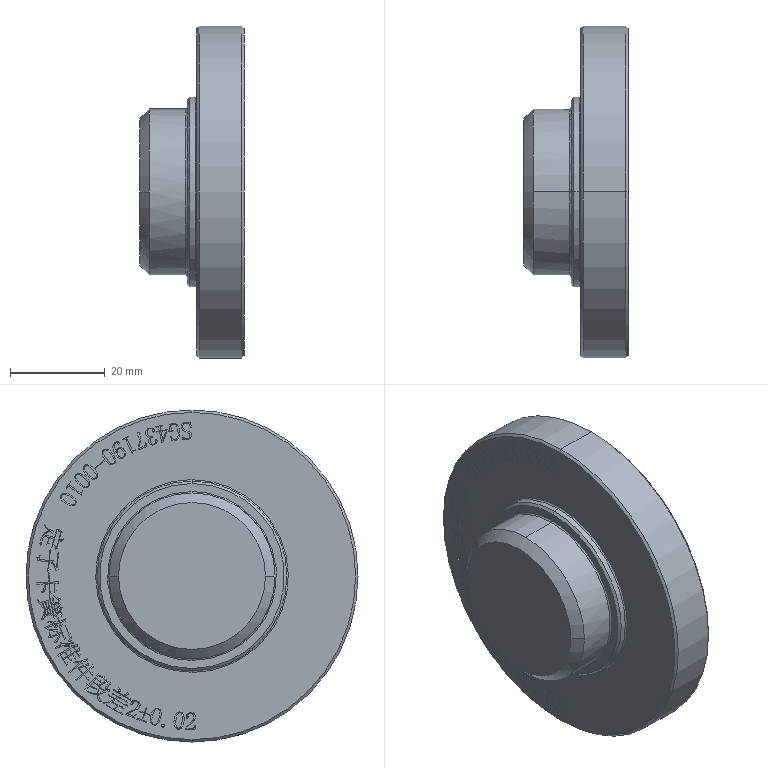Part | STEP file | Stator clip std part | 1 solid | 761 faces | box 22 x 70 x 70 mm | volume 50341 mm3 | plane 491 | spline 256 | cone 8 | cylinder 6 | commonest cylinder face diameters 35 x2 40 x2 70 x2